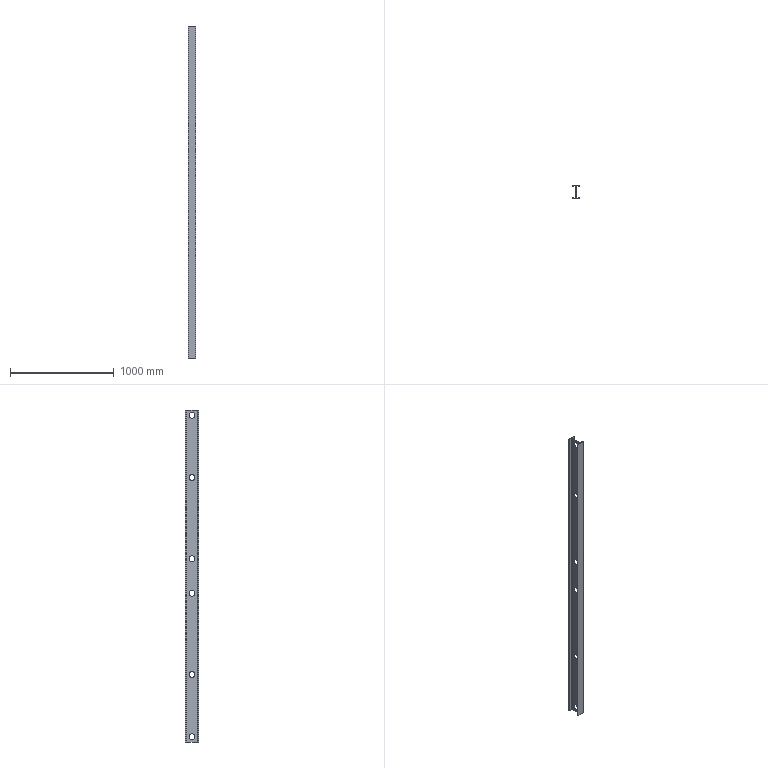Part | SolidWorks | features Extrusion 1, ICE 1 | 1 solid | 30 faces | box 74 x 126 x 3200 mm | volume 4580786 mm3 | cylinder 20 | plane 10 | commonest cylinder face diameters 55 x12 7 x4 14 x4
STEP:
#1=CARTESIAN_POINT('',(-2.5,27.5,2550.));
#2=VERTEX_POINT('',#1);
#3=CARTESIAN_POINT('',(-2.5,-27.5,2550.));
#4=VERTEX_POINT('',#3);
#5=CARTESIAN_POINT('',(-2.5,0.,2550.));
#6=DIRECTION('',(-1.,0.,0.));
#7=DIRECTION('',(0.,0.,-1.));
#8=AXIS2_PLACEMENT_3D('',#5,#6,#7);
#9=CIRCLE('',#8,27.5);
#10=EDGE_CURVE('',#2,#4,#9,.T.);
#11=ORIENTED_EDGE('',*,*,#10,.T.);
#12=CARTESIAN_POINT('',(2.5,-27.5,2550.));
#13=VERTEX_POINT('',#12);
#14=CARTESIAN_POINT('',(-37.001,-27.5,2550.));
#15=DIRECTION('',(1.,0.,0.));
#16=VECTOR('',#15,1000.);
#17=LINE('',#14,#16);
#18=EDGE_CURVE('',#4,#13,#17,.T.);
#19=ORIENTED_EDGE('',*,*,#18,.T.);
#20=CARTESIAN_POINT('',(2.5,27.5,2550.));
#21=VERTEX_POINT('',#20);
#22=CARTESIAN_POINT('',(2.5,0.,2550.));
#23=DIRECTION('',(1.,0.,0.));
#24=DIRECTION('',(0.,1.,0.));
#25=AXIS2_PLACEMENT_3D('',#22,#23,#24);
#26=CIRCLE('',#25,27.5);
#27=EDGE_CURVE('',#13,#21,#26,.T.);
#28=ORIENTED_EDGE('',*,*,#27,.T.);
#29=CARTESIAN_POINT('',(-37.001,27.5,2550.));
#30=DIRECTION('',(1.,0.,0.));
#31=VECTOR('',#30,1000.);
#32=LINE('',#29,#31);
#33=EDGE_CURVE('',#2,#21,#32,.T.);
#34=ORIENTED_EDGE('',*,*,#33,.F.);
#35=EDGE_LOOP('',(#11,#19,#28,#34));
#36=FACE_OUTER_BOUND('',#35,.T.);
#37=CARTESIAN_POINT('',(-37.001,0.,2550.));
#38=DIRECTION('',(1.,0.,0.));
#39=DIRECTION('',(0.,1.,0.));
#40=AXIS2_PLACEMENT_3D('',#37,#38,#39);
#41=CYLINDRICAL_SURFACE('',#40,27.5);
#42=ADVANCED_FACE('',(#36),#41,.F.);
#43=CARTESIAN_POINT('',(-2.5,27.5,3150.));
#44=VERTEX_POINT('',#43);
#45=CARTESIAN_POINT('',(-2.5,-27.5,3150.));
#46=VERTEX_POINT('',#45);
#47=CARTESIAN_POINT('',(-2.5,0.,3150.));
#48=DIRECTION('',(-1.,0.,0.));
#49=DIRECTION('',(0.,0.,-1.));
#50=AXIS2_PLACEMENT_3D('',#47,#48,#49);
#51=CIRCLE('',#50,27.5);
#52=EDGE_CURVE('',#44,#46,#51,.T.);
#53=ORIENTED_EDGE('',*,*,#52,.T.);
#54=CARTESIAN_POINT('',(2.5,-27.5,3150.));
#55=VERTEX_POINT('',#54);
#56=CARTESIAN_POINT('',(-37.001,-27.5,3150.));
#57=DIRECTION('',(1.,0.,0.));
#58=VECTOR('',#57,1000.);
#59=LINE('',#56,#58);
#60=EDGE_CURVE('',#46,#55,#59,.T.);
#61=ORIENTED_EDGE('',*,*,#60,.T.);
#62=CARTESIAN_POINT('',(2.5,27.5,3150.));
#63=VERTEX_POINT('',#62);
#64=CARTESIAN_POINT('',(2.5,0.,3150.));
#65=DIRECTION('',(1.,0.,0.));
#66=DIRECTION('',(0.,1.,0.));
#67=AXIS2_PLACEMENT_3D('',#64,#65,#66);
#68=CIRCLE('',#67,27.5);
#69=EDGE_CURVE('',#55,#63,#68,.T.);
#70=ORIENTED_EDGE('',*,*,#69,.T.);
#71=CARTESIAN_POINT('',(-37.001,27.5,3150.));
#72=DIRECTION('',(1.,0.,0.));
#73=VECTOR('',#72,1000.);
#74=LINE('',#71,#73);
#75=EDGE_CURVE('',#44,#63,#74,.T.);
#76=ORIENTED_EDGE('',*,*,#75,.F.);
#77=EDGE_LOOP('',(#53,#61,#70,#76));
#78=FACE_OUTER_BOUND('',#77,.T.);
#79=CARTESIAN_POINT('',(-37.001,0.,3150.));
#80=DIRECTION('',(1.,0.,0.));
#81=DIRECTION('',(0.,1.,0.));
#82=AXIS2_PLACEMENT_3D('',#79,#80,#81);
#83=CYLINDRICAL_SURFACE('',#82,27.5);
#84=ADVANCED_FACE('',(#78),#83,.F.);
#85=CARTESIAN_POINT('',(-2.5,27.5,1766.));
#86=VERTEX_POINT('',#85);
#87=CARTESIAN_POINT('',(-2.5,-27.5,1766.));
#88=VERTEX_POINT('',#87);
#89=CARTESIAN_POINT('',(-2.5,0.,1766.));
#90=DIRECTION('',(-1.,0.,0.));
#91=DIRECTION('',(0.,0.,-1.));
#92=AXIS2_PLACEMENT_3D('',#89,#90,#91);
#93=CIRCLE('',#92,27.5);
#94=EDGE_CURVE('',#86,#88,#93,.T.);
#95=ORIENTED_EDGE('',*,*,#94,.T.);
#96=CARTESIAN_POINT('',(2.5,-27.5,1766.));
#97=VERTEX_POINT('',#96);
#98=CARTESIAN_POINT('',(-37.001,-27.5,1766.));
#99=DIRECTION('',(1.,0.,0.));
#100=VECTOR('',#99,1000.);
#101=LINE('',#98,#100);
#102=EDGE_CURVE('',#88,#97,#101,.T.);
#103=ORIENTED_EDGE('',*,*,#102,.T.);
#104=CARTESIAN_POINT('',(2.5,27.5,1766.));
#105=VERTEX_POINT('',#104);
#106=CARTESIAN_POINT('',(2.5,0.,1766.));
#107=DIRECTION('',(1.,0.,0.));
#108=DIRECTION('',(0.,1.,0.));
#109=AXIS2_PLACEMENT_3D('',#106,#107,#108);
#110=CIRCLE('',#109,27.5);
#111=EDGE_CURVE('',#97,#105,#110,.T.);
#112=ORIENTED_EDGE('',*,*,#111,.T.);
#113=CARTESIAN_POINT('',(-37.001,27.5,1766.));
#114=DIRECTION('',(1.,0.,0.));
#115=VECTOR('',#114,1000.);
#116=LINE('',#113,#115);
#117=EDGE_CURVE('',#86,#105,#116,.T.);
#118=ORIENTED_EDGE('',*,*,#117,.F.);
#119=EDGE_LOOP('',(#95,#103,#112,#118));
#120=FACE_OUTER_BOUND('',#119,.T.);
#121=CARTESIAN_POINT('',(-37.001,0.,1766.));
#122=DIRECTION('',(1.,0.,0.));
#123=DIRECTION('',(0.,1.,0.));
#124=AXIS2_PLACEMENT_3D('',#121,#122,#123);
#125=CYLINDRICAL_SURFACE('',#124,27.5);
#126=ADVANCED_FACE('',(#120),#125,.F.);
#127=CARTESIAN_POINT('',(-2.5,27.5,1434.));
#128=VERTEX_POINT('',#127);
#129=CARTESIAN_POINT('',(-2.5,-27.5,1434.));
#130=VERTEX_POINT('',#129);
#131=CARTESIAN_POINT('',(-2.5,0.,1434.));
#132=DIRECTION('',(-1.,0.,0.));
#133=DIRECTION('',(0.,0.,-1.));
#134=AXIS2_PLACEMENT_3D('',#131,#132,#133);
#135=CIRCLE('',#134,27.5);
#136=EDGE_CURVE('',#128,#130,#135,.T.);
#137=ORIENTED_EDGE('',*,*,#136,.T.);
#138=CARTESIAN_POINT('',(2.5,-27.5,1434.));
#139=VERTEX_POINT('',#138);
#140=CARTESIAN_POINT('',(-37.001,-27.5,1434.));
#141=DIRECTION('',(1.,0.,0.));
#142=VECTOR('',#141,1000.);
#143=LINE('',#140,#142);
#144=EDGE_CURVE('',#130,#139,#143,.T.);
#145=ORIENTED_EDGE('',*,*,#144,.T.);
#146=CARTESIAN_POINT('',(2.5,27.5,1434.));
#147=VERTEX_POINT('',#146);
#148=CARTESIAN_POINT('',(2.5,0.,1434.));
#149=DIRECTION('',(1.,0.,0.));
#150=DIRECTION('',(0.,1.,0.));
#151=AXIS2_PLACEMENT_3D('',#148,#149,#150);
#152=CIRCLE('',#151,27.5);
#153=EDGE_CURVE('',#139,#147,#152,.T.);
#154=ORIENTED_EDGE('',*,*,#153,.T.);
#155=CARTESIAN_POINT('',(-37.001,27.5,1434.));
#156=DIRECTION('',(1.,0.,0.));
#157=VECTOR('',#156,1000.);
#158=LINE('',#155,#157);
#159=EDGE_CURVE('',#128,#147,#158,.T.);
#160=ORIENTED_EDGE('',*,*,#159,.F.);
#161=EDGE_LOOP('',(#137,#145,#154,#160));
#162=FACE_OUTER_BOUND('',#161,.T.);
#163=CARTESIAN_POINT('',(-37.001,0.,1434.));
#164=DIRECTION('',(1.,0.,0.));
#165=DIRECTION('',(0.,1.,0.));
#166=AXIS2_PLACEMENT_3D('',#163,#164,#165);
#167=CYLINDRICAL_SURFACE('',#166,27.5);
#168=ADVANCED_FACE('',(#162),#167,.F.);
#169=CARTESIAN_POINT('',(-2.5,27.5,650.));
#170=VERTEX_POINT('',#169);
#171=CARTESIAN_POINT('',(-2.5,-27.5,650.));
#172=VERTEX_POINT('',#171);
#173=CARTESIAN_POINT('',(-2.5,0.,650.));
#174=DIRECTION('',(-1.,0.,0.));
#175=DIRECTION('',(0.,0.,-1.));
#176=AXIS2_PLACEMENT_3D('',#173,#174,#175);
#177=CIRCLE('',#176,27.5);
#178=EDGE_CURVE('',#170,#172,#177,.T.);
#179=ORIENTED_EDGE('',*,*,#178,.T.);
#180=CARTESIAN_POINT('',(2.5,-27.5,650.));
#181=VERTEX_POINT('',#180);
#182=CARTESIAN_POINT('',(-37.001,-27.5,650.));
#183=DIRECTION('',(1.,0.,0.));
#184=VECTOR('',#183,1000.);
#185=LINE('',#182,#184);
#186=EDGE_CURVE('',#172,#181,#185,.T.);
#187=ORIENTED_EDGE('',*,*,#186,.T.);
#188=CARTESIAN_POINT('',(2.5,27.5,650.));
#189=VERTEX_POINT('',#188);
#190=CARTESIAN_POINT('',(2.5,0.,650.));
#191=DIRECTION('',(1.,0.,0.));
#192=DIRECTION('',(0.,1.,0.));
#193=AXIS2_PLACEMENT_3D('',#190,#191,#192);
#194=CIRCLE('',#193,27.5);
#195=EDGE_CURVE('',#181,#189,#194,.T.);
#196=ORIENTED_EDGE('',*,*,#195,.T.);
#197=CARTESIAN_POINT('',(-37.001,27.5,650.));
#198=DIRECTION('',(1.,0.,0.));
#199=VECTOR('',#198,1000.);
#200=LINE('',#197,#199);
#201=EDGE_CURVE('',#170,#189,#200,.T.);
#202=ORIENTED_EDGE('',*,*,#201,.F.);
#203=EDGE_LOOP('',(#179,#187,#196,#202));
#204=FACE_OUTER_BOUND('',#203,.T.);
#205=CARTESIAN_POINT('',(-37.001,0.,650.));
#206=DIRECTION('',(1.,0.,0.));
#207=DIRECTION('',(0.,1.,0.));
#208=AXIS2_PLACEMENT_3D('',#205,#206,#207);
#209=CYLINDRICAL_SURFACE('',#208,27.5);
#210=ADVANCED_FACE('',(#204),#209,.F.);
#211=CARTESIAN_POINT('',(-2.5,27.5,50.));
#212=VERTEX_POINT('',#211);
#213=CARTESIAN_POINT('',(-2.5,-27.5,50.));
#214=VERTEX_POINT('',#213);
#215=CARTESIAN_POINT('',(-2.5,0.,50.));
#216=DIRECTION('',(-1.,0.,0.));
#217=DIRECTION('',(0.,0.,-1.));
#218=AXIS2_PLACEMENT_3D('',#215,#216,#217);
#219=CIRCLE('',#218,27.5);
#220=EDGE_CURVE('',#212,#214,#219,.T.);
#221=ORIENTED_EDGE('',*,*,#220,.T.);
#222=CARTESIAN_POINT('',(2.5,-27.5,50.));
#223=VERTEX_POINT('',#222);
#224=CARTESIAN_POINT('',(-37.001,-27.5,50.));
#225=DIRECTION('',(1.,0.,0.));
#226=VECTOR('',#225,1000.);
#227=LINE('',#224,#226);
#228=EDGE_CURVE('',#214,#223,#227,.T.);
#229=ORIENTED_EDGE('',*,*,#228,.T.);
#230=CARTESIAN_POINT('',(2.5,27.5,50.));
#231=VERTEX_POINT('',#230);
#232=CARTESIAN_POINT('',(2.5,0.,50.));
#233=DIRECTION('',(1.,0.,0.));
#234=DIRECTION('',(0.,1.,0.));
#235=AXIS2_PLACEMENT_3D('',#232,#233,#234);
#236=CIRCLE('',#235,27.5);
#237=EDGE_CURVE('',#223,#231,#236,.T.);
#238=ORIENTED_EDGE('',*,*,#237,.T.);
#239=CARTESIAN_POINT('',(-37.001,27.5,50.));
#240=DIRECTION('',(1.,0.,0.));
#241=VECTOR('',#240,1000.);
#242=LINE('',#239,#241);
#243=EDGE_CURVE('',#212,#231,#242,.T.);
#244=ORIENTED_EDGE('',*,*,#243,.F.);
#245=EDGE_LOOP('',(#221,#229,#238,#244));
#246=FACE_OUTER_BOUND('',#245,.T.);
#247=CARTESIAN_POINT('',(-37.001,0.,50.));
#248=DIRECTION('',(1.,0.,0.));
#249=DIRECTION('',(0.,1.,0.));
#250=AXIS2_PLACEMENT_3D('',#247,#248,#249);
#251=CYLINDRICAL_SURFACE('',#250,27.5);
#252=ADVANCED_FACE('',(#246),#251,.F.);
#253=CARTESIAN_POINT('',(-2.5,-48.4,0.));
#254=VERTEX_POINT('',#253);
#255=CARTESIAN_POINT('',(-8.361,-55.307,0.));
#256=VERTEX_POINT('',#255);
#257=CARTESIAN_POINT('',(-9.5,-48.4,0.));
#258=DIRECTION('',(0.,0.,-1.));
#259=DIRECTION('',(-1.,0.,0.));
#260=AXIS2_PLACEMENT_3D('',#257,#258,#259);
#261=CIRCLE('',#260,7.);
#262=EDGE_CURVE('',#254,#256,#261,.T.);
#263=ORIENTED_EDGE('',*,*,#262,.T.);
#264=CARTESIAN_POINT('',(-8.361,-55.307,3200.));
#265=VERTEX_POINT('',#264);
#266=CARTESIAN_POINT('',(-8.361,-55.307,3200.));
#267=DIRECTION('',(0.,0.,-1.));
#268=VECTOR('',#267,1000.);
#269=LINE('',#266,#268);
#270=EDGE_CURVE('',#265,#256,#269,.T.);
#271=ORIENTED_EDGE('',*,*,#270,.F.);
#272=CARTESIAN_POINT('',(-2.5,-48.4,3200.));
#273=VERTEX_POINT('',#272);
#274=CARTESIAN_POINT('',(-9.5,-48.4,3200.));
#275=DIRECTION('',(0.,0.,-1.));
#276=DIRECTION('',(-1.,0.,0.));
#277=AXIS2_PLACEMENT_3D('',#274,#275,#276);
#278=CIRCLE('',#277,7.);
#279=EDGE_CURVE('',#273,#265,#278,.T.);
#280=ORIENTED_EDGE('',*,*,#279,.F.);
#281=CARTESIAN_POINT('',(-2.5,-48.4,3200.));
#282=DIRECTION('',(0.,0.,-1.));
#283=VECTOR('',#282,1000.);
#284=LINE('',#281,#283);
#285=EDGE_CURVE('',#273,#254,#284,.T.);
#286=ORIENTED_EDGE('',*,*,#285,.T.);
#287=EDGE_LOOP('',(#263,#271,#280,#286));
#288=FACE_OUTER_BOUND('',#287,.T.);
#289=CARTESIAN_POINT('',(-9.5,-48.4,3200.));
#290=DIRECTION('',(0.,0.,-1.));
#291=DIRECTION('',(-1.,0.,0.));
#292=AXIS2_PLACEMENT_3D('',#289,#290,#291);
#293=CYLINDRICAL_SURFACE('',#292,7.);
#294=ADVANCED_FACE('',(#288),#293,.F.);
#295=CARTESIAN_POINT('',(-34.07,-59.547,0.));
#296=VERTEX_POINT('',#295);
#297=CARTESIAN_POINT('',(-34.07,-59.547,0.));
#298=DIRECTION('',(-0.9867,-0.1627,0.));
#299=VECTOR('',#298,1000.);
#300=LINE('',#297,#299);
#301=EDGE_CURVE('',#256,#296,#300,.T.);
#302=ORIENTED_EDGE('',*,*,#301,.T.);
#303=CARTESIAN_POINT('',(-34.07,-59.547,3200.));
#304=VERTEX_POINT('',#303);
#305=CARTESIAN_POINT('',(-34.07,-59.547,3200.));
#306=DIRECTION('',(0.,0.,-1.));
#307=VECTOR('',#306,1000.);
#308=LINE('',#305,#307);
#309=EDGE_CURVE('',#304,#296,#308,.T.);
#310=ORIENTED_EDGE('',*,*,#309,.F.);
#311=CARTESIAN_POINT('',(-34.07,-59.547,3200.));
#312=DIRECTION('',(-0.9867,-0.1627,0.));
#313=VECTOR('',#312,1000.);
#314=LINE('',#311,#313);
#315=EDGE_CURVE('',#265,#304,#314,.T.);
#316=ORIENTED_EDGE('',*,*,#315,.F.);
#317=ORIENTED_EDGE('',*,*,#270,.T.);
#318=EDGE_LOOP('',(#302,#310,#316,#317));
#319=FACE_OUTER_BOUND('',#318,.T.);
#320=CARTESIAN_POINT('',(-34.07,-59.547,3200.));
#321=DIRECTION('',(0.1627,-0.9867,0.));
#322=DIRECTION('',(0.9867,0.1627,0.));
#323=AXIS2_PLACEMENT_3D('',#320,#321,#322);
#324=PLANE('',#323);
#325=ADVANCED_FACE('',(#319),#324,.F.);
#326=CARTESIAN_POINT('',(-37.,-63.,0.));
#327=VERTEX_POINT('',#326);
#328=CARTESIAN_POINT('',(-33.5,-63.,0.));
#329=DIRECTION('',(0.,0.,1.));
#330=DIRECTION('',(-1.,0.,0.));
#331=AXIS2_PLACEMENT_3D('',#328,#329,#330);
#332=CIRCLE('',#331,3.5);
#333=EDGE_CURVE('',#296,#327,#332,.T.);
#334=ORIENTED_EDGE('',*,*,#333,.T.);
#335=CARTESIAN_POINT('',(-37.,-63.,3200.));
#336=VERTEX_POINT('',#335);
#337=CARTESIAN_POINT('',(-37.,-63.,3200.));
#338=DIRECTION('',(0.,0.,-1.));
#339=VECTOR('',#338,1000.);
#340=LINE('',#337,#339);
#341=EDGE_CURVE('',#336,#327,#340,.T.);
#342=ORIENTED_EDGE('',*,*,#341,.F.);
#343=CARTESIAN_POINT('',(-33.5,-63.,3200.));
#344=DIRECTION('',(0.,0.,1.));
#345=DIRECTION('',(-1.,0.,0.));
#346=AXIS2_PLACEMENT_3D('',#343,#344,#345);
#347=CIRCLE('',#346,3.5);
#348=EDGE_CURVE('',#304,#336,#347,.T.);
#349=ORIENTED_EDGE('',*,*,#348,.F.);
#350=ORIENTED_EDGE('',*,*,#309,.T.);
#351=EDGE_LOOP('',(#334,#342,#349,#350));
#352=FACE_OUTER_BOUND('',#351,.T.);
#353=CARTESIAN_POINT('',(-33.5,-63.,3200.));
#354=DIRECTION('',(0.,0.,-1.));
#355=DIRECTION('',(-1.,0.,0.));
#356=AXIS2_PLACEMENT_3D('',#353,#354,#355);
#357=CYLINDRICAL_SURFACE('',#356,3.5);
#358=ADVANCED_FACE('',(#352),#357,.T.);
#359=CARTESIAN_POINT('',(37.,-63.,0.));
#360=VERTEX_POINT('',#359);
#361=CARTESIAN_POINT('',(-37.,-63.,0.));
#362=DIRECTION('',(1.,0.,0.));
#363=VECTOR('',#362,1000.);
#364=LINE('',#361,#363);
#365=EDGE_CURVE('',#327,#360,#364,.T.);
#366=ORIENTED_EDGE('',*,*,#365,.T.);
#367=CARTESIAN_POINT('',(37.,-63.,3200.));
#368=VERTEX_POINT('',#367);
#369=CARTESIAN_POINT('',(37.,-63.,3200.));
#370=DIRECTION('',(0.,0.,-1.));
#371=VECTOR('',#370,1000.);
#372=LINE('',#369,#371);
#373=EDGE_CURVE('',#368,#360,#372,.T.);
#374=ORIENTED_EDGE('',*,*,#373,.F.);
#375=CARTESIAN_POINT('',(-37.,-63.,3200.));
#376=DIRECTION('',(1.,0.,0.));
#377=VECTOR('',#376,1000.);
#378=LINE('',#375,#377);
#379=EDGE_CURVE('',#336,#368,#378,.T.);
#380=ORIENTED_EDGE('',*,*,#379,.F.);
#381=ORIENTED_EDGE('',*,*,#341,.T.);
#382=EDGE_LOOP('',(#366,#374,#380,#381));
#383=FACE_OUTER_BOUND('',#382,.T.);
#384=CARTESIAN_POINT('',(-37.,-63.,3200.));
#385=DIRECTION('',(0.,1.,0.));
#386=DIRECTION('',(0.,0.,1.));
#387=AXIS2_PLACEMENT_3D('',#384,#385,#386);
#388=PLANE('',#387);
#389=ADVANCED_FACE('',(#383),#388,.F.);
#390=CARTESIAN_POINT('',(34.07,-59.547,0.));
#391=VERTEX_POINT('',#390);
#392=CARTESIAN_POINT('',(33.5,-63.,0.));
#393=DIRECTION('',(0.,0.,1.));
#394=DIRECTION('',(1.,0.,0.));
#395=AXIS2_PLACEMENT_3D('',#392,#393,#394);
#396=CIRCLE('',#395,3.5);
#397=EDGE_CURVE('',#360,#391,#396,.T.);
#398=ORIENTED_EDGE('',*,*,#397,.T.);
#399=CARTESIAN_POINT('',(34.07,-59.547,3200.));
#400=VERTEX_POINT('',#399);
#401=CARTESIAN_POINT('',(34.07,-59.547,3200.));
#402=DIRECTION('',(0.,0.,-1.));
#403=VECTOR('',#402,1000.);
#404=LINE('',#401,#403);
#405=EDGE_CURVE('',#400,#391,#404,.T.);
#406=ORIENTED_EDGE('',*,*,#405,.F.);
#407=CARTESIAN_POINT('',(33.5,-63.,3200.));
#408=DIRECTION('',(0.,0.,1.));
#409=DIRECTION('',(1.,0.,0.));
#410=AXIS2_PLACEMENT_3D('',#407,#408,#409);
#411=CIRCLE('',#410,3.5);
#412=EDGE_CURVE('',#368,#400,#411,.T.);
#413=ORIENTED_EDGE('',*,*,#412,.F.);
#414=ORIENTED_EDGE('',*,*,#373,.T.);
#415=EDGE_LOOP('',(#398,#406,#413,#414));
#416=FACE_OUTER_BOUND('',#415,.T.);
#417=CARTESIAN_POINT('',(33.5,-63.,3200.));
#418=DIRECTION('',(0.,0.,-1.));
#419=DIRECTION('',(-1.,0.,0.));
#420=AXIS2_PLACEMENT_3D('',#417,#418,#419);
#421=CYLINDRICAL_SURFACE('',#420,3.5);
#422=ADVANCED_FACE('',(#416),#421,.T.);
#423=CARTESIAN_POINT('',(8.361,-55.307,0.));
#424=VERTEX_POINT('',#423);
#425=CARTESIAN_POINT('',(34.07,-59.547,0.));
#426=DIRECTION('',(-0.9867,0.1627,0.));
#427=VECTOR('',#426,1000.);
#428=LINE('',#425,#427);
#429=EDGE_CURVE('',#391,#424,#428,.T.);
#430=ORIENTED_EDGE('',*,*,#429,.T.);
#431=CARTESIAN_POINT('',(8.361,-55.307,3200.));
#432=VERTEX_POINT('',#431);
#433=CARTESIAN_POINT('',(8.361,-55.307,3200.));
#434=DIRECTION('',(0.,0.,-1.));
#435=VECTOR('',#434,1000.);
#436=LINE('',#433,#435);
#437=EDGE_CURVE('',#432,#424,#436,.T.);
#438=ORIENTED_EDGE('',*,*,#437,.F.);
#439=CARTESIAN_POINT('',(34.07,-59.547,3200.));
#440=DIRECTION('',(-0.9867,0.1627,0.));
#441=VECTOR('',#440,1000.);
#442=LINE('',#439,#441);
#443=EDGE_CURVE('',#400,#432,#442,.T.);
#444=ORIENTED_EDGE('',*,*,#443,.F.);
#445=ORIENTED_EDGE('',*,*,#405,.T.);
#446=EDGE_LOOP('',(#430,#438,#444,#445));
#447=FACE_OUTER_BOUND('',#446,.T.);
#448=CARTESIAN_POINT('',(34.07,-59.547,3200.));
#449=DIRECTION('',(-0.1627,-0.9867,0.));
#450=DIRECTION('',(0.9867,-0.1627,0.));
#451=AXIS2_PLACEMENT_3D('',#448,#449,#450);
#452=PLANE('',#451);
#453=ADVANCED_FACE('',(#447),#452,.F.);
#454=CARTESIAN_POINT('',(2.5,-48.4,0.));
#455=VERTEX_POINT('',#454);
#456=CARTESIAN_POINT('',(9.5,-48.4,0.));
#457=DIRECTION('',(0.,0.,-1.));
#458=DIRECTION('',(1.,0.,0.));
#459=AXIS2_PLACEMENT_3D('',#456,#457,#458);
#460=CIRCLE('',#459,7.);
#461=EDGE_CURVE('',#424,#455,#460,.T.);
#462=ORIENTED_EDGE('',*,*,#461,.T.);
#463=CARTESIAN_POINT('',(2.5,-48.4,3200.));
#464=VERTEX_POINT('',#463);
#465=CARTESIAN_POINT('',(2.5,-48.4,3200.));
#466=DIRECTION('',(0.,0.,-1.));
#467=VECTOR('',#466,1000.);
#468=LINE('',#465,#467);
#469=EDGE_CURVE('',#464,#455,#468,.T.);
#470=ORIENTED_EDGE('',*,*,#469,.F.);
#471=CARTESIAN_POINT('',(9.5,-48.4,3200.));
#472=DIRECTION('',(0.,0.,-1.));
#473=DIRECTION('',(1.,0.,0.));
#474=AXIS2_PLACEMENT_3D('',#471,#472,#473);
#475=CIRCLE('',#474,7.);
#476=EDGE_CURVE('',#432,#464,#475,.T.);
#477=ORIENTED_EDGE('',*,*,#476,.F.);
#478=ORIENTED_EDGE('',*,*,#437,.T.);
#479=EDGE_LOOP('',(#462,#470,#477,#478));
#480=FACE_OUTER_BOUND('',#479,.T.);
#481=CARTESIAN_POINT('',(9.5,-48.4,3200.));
#482=DIRECTION('',(0.,0.,-1.));
#483=DIRECTION('',(-1.,0.,0.));
#484=AXIS2_PLACEMENT_3D('',#481,#482,#483);
#485=CYLINDRICAL_SURFACE('',#484,7.);
#486=ADVANCED_FACE('',(#480),#485,.F.);
#487=CARTESIAN_POINT('',(2.5,0.,2550.));
#488=DIRECTION('',(1.,0.,0.));
#489=DIRECTION('',(0.,1.,0.));
#490=AXIS2_PLACEMENT_3D('',#487,#488,#489);
#491=CIRCLE('',#490,27.5);
#492=EDGE_CURVE('',#21,#13,#491,.T.);
#493=ORIENTED_EDGE('',*,*,#492,.F.);
#494=ORIENTED_EDGE('',*,*,#27,.F.);
#495=EDGE_LOOP('',(#493,#494));
#496=FACE_BOUND('',#495,.T.);
#497=CARTESIAN_POINT('',(2.5,0.,3150.));
#498=DIRECTION('',(1.,0.,0.));
#499=DIRECTION('',(0.,1.,0.));
#500=AXIS2_PLACEMENT_3D('',#497,#498,#499);
#501=CIRCLE('',#500,27.5);
#502=EDGE_CURVE('',#63,#55,#501,.T.);
#503=ORIENTED_EDGE('',*,*,#502,.F.);
#504=ORIENTED_EDGE('',*,*,#69,.F.);
#505=EDGE_LOOP('',(#503,#504));
#506=FACE_BOUND('',#505,.T.);
#507=CARTESIAN_POINT('',(2.5,0.,1766.));
#508=DIRECTION('',(1.,0.,0.));
#509=DIRECTION('',(0.,1.,0.));
#510=AXIS2_PLACEMENT_3D('',#507,#508,#509);
#511=CIRCLE('',#510,27.5);
#512=EDGE_CURVE('',#105,#97,#511,.T.);
#513=ORIENTED_EDGE('',*,*,#512,.F.);
#514=ORIENTED_EDGE('',*,*,#111,.F.);
#515=EDGE_LOOP('',(#513,#514));
#516=FACE_BOUND('',#515,.T.);
#517=CARTESIAN_POINT('',(2.5,0.,1434.));
#518=DIRECTION('',(1.,0.,0.));
#519=DIRECTION('',(0.,1.,0.));
#520=AXIS2_PLACEMENT_3D('',#517,#518,#519);
#521=CIRCLE('',#520,27.5);
#522=EDGE_CURVE('',#147,#139,#521,.T.);
#523=ORIENTED_EDGE('',*,*,#522,.F.);
#524=ORIENTED_EDGE('',*,*,#153,.F.);
#525=EDGE_LOOP('',(#523,#524));
#526=FACE_BOUND('',#525,.T.);
#527=CARTESIAN_POINT('',(2.5,0.,650.));
#528=DIRECTION('',(1.,0.,0.));
#529=DIRECTION('',(0.,1.,0.));
#530=AXIS2_PLACEMENT_3D('',#527,#528,#529);
#531=CIRCLE('',#530,27.5);
#532=EDGE_CURVE('',#189,#181,#531,.T.);
#533=ORIENTED_EDGE('',*,*,#532,.F.);
#534=ORIENTED_EDGE('',*,*,#195,.F.);
#535=EDGE_LOOP('',(#533,#534));
#536=FACE_BOUND('',#535,.T.);
#537=CARTESIAN_POINT('',(2.5,0.,50.));
#538=DIRECTION('',(1.,0.,0.));
#539=DIRECTION('',(0.,1.,0.));
#540=AXIS2_PLACEMENT_3D('',#537,#538,#539);
#541=CIRCLE('',#540,27.5);
#542=EDGE_CURVE('',#231,#223,#541,.T.);
#543=ORIENTED_EDGE('',*,*,#542,.F.);
#544=ORIENTED_EDGE('',*,*,#237,.F.);
#545=EDGE_LOOP('',(#543,#544));
#546=FACE_BOUND('',#545,.T.);
#547=CARTESIAN_POINT('',(2.5,48.4,0.));
#548=VERTEX_POINT('',#547);
#549=CARTESIAN_POINT('',(2.5,48.4,0.));
#550=DIRECTION('',(0.,1.,0.));
#551=VECTOR('',#550,1000.);
#552=LINE('',#549,#551);
#553=EDGE_CURVE('',#455,#548,#552,.T.);
#554=ORIENTED_EDGE('',*,*,#553,.T.);
#555=CARTESIAN_POINT('',(2.5,48.4,3200.));
#556=VERTEX_POINT('',#555);
#557=CARTESIAN_POINT('',(2.5,48.4,3200.));
#558=DIRECTION('',(0.,0.,-1.));
#559=VECTOR('',#558,1000.);
#560=LINE('',#557,#559);
#561=EDGE_CURVE('',#556,#548,#560,.T.);
#562=ORIENTED_EDGE('',*,*,#561,.F.);
#563=CARTESIAN_POINT('',(2.5,48.4,3200.));
#564=DIRECTION('',(0.,1.,0.));
#565=VECTOR('',#564,1000.);
#566=LINE('',#563,#565);
#567=EDGE_CURVE('',#464,#556,#566,.T.);
#568=ORIENTED_EDGE('',*,*,#567,.F.);
#569=ORIENTED_EDGE('',*,*,#469,.T.);
#570=EDGE_LOOP('',(#554,#562,#568,#569));
#571=FACE_OUTER_BOUND('',#570,.T.);
#572=CARTESIAN_POINT('',(2.5,48.4,3200.));
#573=DIRECTION('',(-1.,0.,0.));
#574=DIRECTION('',(0.,-1.,0.));
#575=AXIS2_PLACEMENT_3D('',#572,#573,#574);
#576=PLANE('',#575);
#577=ADVANCED_FACE('',(#496,#506,#516,#526,#536,#546,#571),#576,.F.);
#578=CARTESIAN_POINT('',(8.361,55.307,0.));
#579=VERTEX_POINT('',#578);
#580=CARTESIAN_POINT('',(9.5,48.4,0.));
#581=DIRECTION('',(0.,0.,-1.));
#582=DIRECTION('',(-1.,0.,0.));
#583=AXIS2_PLACEMENT_3D('',#580,#581,#582);
#584=CIRCLE('',#583,7.);
#585=EDGE_CURVE('',#548,#579,#584,.T.);
#586=ORIENTED_EDGE('',*,*,#585,.T.);
#587=CARTESIAN_POINT('',(8.361,55.307,3200.));
#588=VERTEX_POINT('',#587);
#589=CARTESIAN_POINT('',(8.361,55.307,3200.));
#590=DIRECTION('',(0.,0.,-1.));
#591=VECTOR('',#590,1000.);
#592=LINE('',#589,#591);
#593=EDGE_CURVE('',#588,#579,#592,.T.);
#594=ORIENTED_EDGE('',*,*,#593,.F.);
#595=CARTESIAN_POINT('',(9.5,48.4,3200.));
#596=DIRECTION('',(0.,0.,-1.));
#597=DIRECTION('',(-1.,0.,0.));
#598=AXIS2_PLACEMENT_3D('',#595,#596,#597);
#599=CIRCLE('',#598,7.);
#600=EDGE_CURVE('',#556,#588,#599,.T.);
#601=ORIENTED_EDGE('',*,*,#600,.F.);
#602=ORIENTED_EDGE('',*,*,#561,.T.);
#603=EDGE_LOOP('',(#586,#594,#601,#602));
#604=FACE_OUTER_BOUND('',#603,.T.);
#605=CARTESIAN_POINT('',(9.5,48.4,3200.));
#606=DIRECTION('',(0.,0.,-1.));
#607=DIRECTION('',(-1.,0.,0.));
#608=AXIS2_PLACEMENT_3D('',#605,#606,#607);
#609=CYLINDRICAL_SURFACE('',#608,7.);
#610=ADVANCED_FACE('',(#604),#609,.F.);
#611=CARTESIAN_POINT('',(34.07,59.547,0.));
#612=VERTEX_POINT('',#611);
#613=CARTESIAN_POINT('',(34.07,59.547,0.));
#614=DIRECTION('',(0.9867,0.1627,0.));
#615=VECTOR('',#614,1000.);
#616=LINE('',#613,#615);
#617=EDGE_CURVE('',#579,#612,#616,.T.);
#618=ORIENTED_EDGE('',*,*,#617,.T.);
#619=CARTESIAN_POINT('',(34.07,59.547,3200.));
#620=VERTEX_POINT('',#619);
#621=CARTESIAN_POINT('',(34.07,59.547,3200.));
#622=DIRECTION('',(0.,0.,-1.));
#623=VECTOR('',#622,1000.);
#624=LINE('',#621,#623);
#625=EDGE_CURVE('',#620,#612,#624,.T.);
#626=ORIENTED_EDGE('',*,*,#625,.F.);
#627=CARTESIAN_POINT('',(34.07,59.547,3200.));
#628=DIRECTION('',(0.9867,0.1627,0.));
#629=VECTOR('',#628,1000.);
#630=LINE('',#627,#629);
#631=EDGE_CURVE('',#588,#620,#630,.T.);
#632=ORIENTED_EDGE('',*,*,#631,.F.);
#633=ORIENTED_EDGE('',*,*,#593,.T.);
#634=EDGE_LOOP('',(#618,#626,#632,#633));
#635=FACE_OUTER_BOUND('',#634,.T.);
#636=CARTESIAN_POINT('',(34.07,59.547,3200.));
#637=DIRECTION('',(-0.1627,0.9867,0.));
#638=DIRECTION('',(-0.9867,-0.1627,0.));
#639=AXIS2_PLACEMENT_3D('',#636,#637,#638);
#640=PLANE('',#639);
#641=ADVANCED_FACE('',(#635),#640,.F.);
#642=CARTESIAN_POINT('',(37.,63.,0.));
#643=VERTEX_POINT('',#642);
#644=CARTESIAN_POINT('',(33.5,63.,0.));
#645=DIRECTION('',(0.,0.,1.));
#646=DIRECTION('',(-1.,0.,0.));
#647=AXIS2_PLACEMENT_3D('',#644,#645,#646);
#648=CIRCLE('',#647,3.5);
#649=EDGE_CURVE('',#612,#643,#648,.T.);
#650=ORIENTED_EDGE('',*,*,#649,.T.);
#651=CARTESIAN_POINT('',(37.,63.,3200.));
#652=VERTEX_POINT('',#651);
#653=CARTESIAN_POINT('',(37.,63.,3200.));
#654=DIRECTION('',(0.,0.,-1.));
#655=VECTOR('',#654,1000.);
#656=LINE('',#653,#655);
#657=EDGE_CURVE('',#652,#643,#656,.T.);
#658=ORIENTED_EDGE('',*,*,#657,.F.);
#659=CARTESIAN_POINT('',(33.5,63.,3200.));
#660=DIRECTION('',(0.,0.,1.));
#661=DIRECTION('',(-1.,0.,0.));
#662=AXIS2_PLACEMENT_3D('',#659,#660,#661);
#663=CIRCLE('',#662,3.5);
#664=EDGE_CURVE('',#620,#652,#663,.T.);
#665=ORIENTED_EDGE('',*,*,#664,.F.);
#666=ORIENTED_EDGE('',*,*,#625,.T.);
#667=EDGE_LOOP('',(#650,#658,#665,#666));
#668=FACE_OUTER_BOUND('',#667,.T.);
#669=CARTESIAN_POINT('',(33.5,63.,3200.));
#670=DIRECTION('',(0.,0.,-1.));
#671=DIRECTION('',(-1.,0.,0.));
#672=AXIS2_PLACEMENT_3D('',#669,#670,#671);
#673=CYLINDRICAL_SURFACE('',#672,3.5);
#674=ADVANCED_FACE('',(#668),#673,.T.);
#675=CARTESIAN_POINT('',(-37.,63.,0.));
#676=VERTEX_POINT('',#675);
#677=CARTESIAN_POINT('',(-37.,63.,0.));
#678=DIRECTION('',(-1.,0.,0.));
#679=VECTOR('',#678,1000.);
#680=LINE('',#677,#679);
#681=EDGE_CURVE('',#643,#676,#680,.T.);
#682=ORIENTED_EDGE('',*,*,#681,.T.);
#683=CARTESIAN_POINT('',(-37.,63.,3200.));
#684=VERTEX_POINT('',#683);
#685=CARTESIAN_POINT('',(-37.,63.,3200.));
#686=DIRECTION('',(0.,0.,-1.));
#687=VECTOR('',#686,1000.);
#688=LINE('',#685,#687);
#689=EDGE_CURVE('',#684,#676,#688,.T.);
#690=ORIENTED_EDGE('',*,*,#689,.F.);
#691=CARTESIAN_POINT('',(-37.,63.,3200.));
#692=DIRECTION('',(-1.,0.,0.));
#693=VECTOR('',#692,1000.);
#694=LINE('',#691,#693);
#695=EDGE_CURVE('',#652,#684,#694,.T.);
#696=ORIENTED_EDGE('',*,*,#695,.F.);
#697=ORIENTED_EDGE('',*,*,#657,.T.);
#698=EDGE_LOOP('',(#682,#690,#696,#697));
#699=FACE_OUTER_BOUND('',#698,.T.);
#700=CARTESIAN_POINT('',(-37.,63.,3200.));
#701=DIRECTION('',(0.,-1.,0.));
#702=DIRECTION('',(0.,0.,-1.));
#703=AXIS2_PLACEMENT_3D('',#700,#701,#702);
#704=PLANE('',#703);
#705=ADVANCED_FACE('',(#699),#704,.F.);
#706=CARTESIAN_POINT('',(-34.07,59.547,0.));
#707=VERTEX_POINT('',#706);
#708=CARTESIAN_POINT('',(-33.5,63.,0.));
#709=DIRECTION('',(0.,0.,1.));
#710=DIRECTION('',(1.,0.,0.));
#711=AXIS2_PLACEMENT_3D('',#708,#709,#710);
#712=CIRCLE('',#711,3.5);
#713=EDGE_CURVE('',#676,#707,#712,.T.);
#714=ORIENTED_EDGE('',*,*,#713,.T.);
#715=CARTESIAN_POINT('',(-34.07,59.547,3200.));
#716=VERTEX_POINT('',#715);
#717=CARTESIAN_POINT('',(-34.07,59.547,3200.));
#718=DIRECTION('',(0.,0.,-1.));
#719=VECTOR('',#718,1000.);
#720=LINE('',#717,#719);
#721=EDGE_CURVE('',#716,#707,#720,.T.);
#722=ORIENTED_EDGE('',*,*,#721,.F.);
#723=CARTESIAN_POINT('',(-33.5,63.,3200.));
#724=DIRECTION('',(0.,0.,1.));
#725=DIRECTION('',(1.,0.,0.));
#726=AXIS2_PLACEMENT_3D('',#723,#724,#725);
#727=CIRCLE('',#726,3.5);
#728=EDGE_CURVE('',#684,#716,#727,.T.);
#729=ORIENTED_EDGE('',*,*,#728,.F.);
#730=ORIENTED_EDGE('',*,*,#689,.T.);
#731=EDGE_LOOP('',(#714,#722,#729,#730));
#732=FACE_OUTER_BOUND('',#731,.T.);
#733=CARTESIAN_POINT('',(-33.5,63.,3200.));
#734=DIRECTION('',(0.,0.,-1.));
#735=DIRECTION('',(-1.,0.,0.));
#736=AXIS2_PLACEMENT_3D('',#733,#734,#735);
#737=CYLINDRICAL_SURFACE('',#736,3.5);
#738=ADVANCED_FACE('',(#732),#737,.T.);
#739=CARTESIAN_POINT('',(-8.361,55.307,0.));
#740=VERTEX_POINT('',#739);
#741=CARTESIAN_POINT('',(-34.07,59.547,0.));
#742=DIRECTION('',(0.9867,-0.1627,0.));
#743=VECTOR('',#742,1000.);
#744=LINE('',#741,#743);
#745=EDGE_CURVE('',#707,#740,#744,.T.);
#746=ORIENTED_EDGE('',*,*,#745,.T.);
#747=CARTESIAN_POINT('',(-8.361,55.307,3200.));
#748=VERTEX_POINT('',#747);
#749=CARTESIAN_POINT('',(-8.361,55.307,3200.));
#750=DIRECTION('',(0.,0.,-1.));
#751=VECTOR('',#750,1000.);
#752=LINE('',#749,#751);
#753=EDGE_CURVE('',#748,#740,#752,.T.);
#754=ORIENTED_EDGE('',*,*,#753,.F.);
#755=CARTESIAN_POINT('',(-34.07,59.547,3200.));
#756=DIRECTION('',(0.9867,-0.1627,0.));
#757=VECTOR('',#756,1000.);
#758=LINE('',#755,#757);
#759=EDGE_CURVE('',#716,#748,#758,.T.);
#760=ORIENTED_EDGE('',*,*,#759,.F.);
#761=ORIENTED_EDGE('',*,*,#721,.T.);
#762=EDGE_LOOP('',(#746,#754,#760,#761));
#763=FACE_OUTER_BOUND('',#762,.T.);
#764=CARTESIAN_POINT('',(-34.07,59.547,3200.));
#765=DIRECTION('',(0.1627,0.9867,0.));
#766=DIRECTION('',(-0.9867,0.1627,0.));
#767=AXIS2_PLACEMENT_3D('',#764,#765,#766);
#768=PLANE('',#767);
#769=ADVANCED_FACE('',(#763),#768,.F.);
#770=CARTESIAN_POINT('',(-2.5,48.4,0.));
#771=VERTEX_POINT('',#770);
#772=CARTESIAN_POINT('',(-9.5,48.4,0.));
#773=DIRECTION('',(0.,0.,-1.));
#774=DIRECTION('',(1.,0.,0.));
#775=AXIS2_PLACEMENT_3D('',#772,#773,#774);
#776=CIRCLE('',#775,7.);
#777=EDGE_CURVE('',#740,#771,#776,.T.);
#778=ORIENTED_EDGE('',*,*,#777,.T.);
#779=CARTESIAN_POINT('',(-2.5,48.4,3200.));
#780=VERTEX_POINT('',#779);
#781=CARTESIAN_POINT('',(-2.5,48.4,3200.));
#782=DIRECTION('',(0.,0.,-1.));
#783=VECTOR('',#782,1000.);
#784=LINE('',#781,#783);
#785=EDGE_CURVE('',#780,#771,#784,.T.);
#786=ORIENTED_EDGE('',*,*,#785,.F.);
#787=CARTESIAN_POINT('',(-9.5,48.4,3200.));
#788=DIRECTION('',(0.,0.,-1.));
#789=DIRECTION('',(1.,0.,0.));
#790=AXIS2_PLACEMENT_3D('',#787,#788,#789);
#791=CIRCLE('',#790,7.);
#792=EDGE_CURVE('',#748,#780,#791,.T.);
#793=ORIENTED_EDGE('',*,*,#792,.F.);
#794=ORIENTED_EDGE('',*,*,#753,.T.);
#795=EDGE_LOOP('',(#778,#786,#793,#794));
#796=FACE_OUTER_BOUND('',#795,.T.);
#797=CARTESIAN_POINT('',(-9.5,48.4,3200.));
#798=DIRECTION('',(0.,0.,-1.));
#799=DIRECTION('',(-1.,0.,0.));
#800=AXIS2_PLACEMENT_3D('',#797,#798,#799);
#801=CYLINDRICAL_SURFACE('',#800,7.);
#802=ADVANCED_FACE('',(#796),#801,.F.);
#803=ORIENTED_EDGE('',*,*,#10,.F.);
#804=CARTESIAN_POINT('',(-2.5,0.,2550.));
#805=DIRECTION('',(-1.,0.,0.));
#806=DIRECTION('',(0.,0.,-1.));
#807=AXIS2_PLACEMENT_3D('',#804,#805,#806);
#808=CIRCLE('',#807,27.5);
#809=EDGE_CURVE('',#4,#2,#808,.T.);
#810=ORIENTED_EDGE('',*,*,#809,.F.);
#811=EDGE_LOOP('',(#803,#810));
#812=FACE_BOUND('',#811,.T.);
#813=ORIENTED_EDGE('',*,*,#52,.F.);
#814=CARTESIAN_POINT('',(-2.5,0.,3150.));
#815=DIRECTION('',(-1.,0.,0.));
#816=DIRECTION('',(0.,0.,-1.));
#817=AXIS2_PLACEMENT_3D('',#814,#815,#816);
#818=CIRCLE('',#817,27.5);
#819=EDGE_CURVE('',#46,#44,#818,.T.);
#820=ORIENTED_EDGE('',*,*,#819,.F.);
#821=EDGE_LOOP('',(#813,#820));
#822=FACE_BOUND('',#821,.T.);
#823=ORIENTED_EDGE('',*,*,#94,.F.);
#824=CARTESIAN_POINT('',(-2.5,0.,1766.));
#825=DIRECTION('',(-1.,0.,0.));
#826=DIRECTION('',(0.,0.,-1.));
#827=AXIS2_PLACEMENT_3D('',#824,#825,#826);
#828=CIRCLE('',#827,27.5);
#829=EDGE_CURVE('',#88,#86,#828,.T.);
#830=ORIENTED_EDGE('',*,*,#829,.F.);
#831=EDGE_LOOP('',(#823,#830));
#832=FACE_BOUND('',#831,.T.);
#833=ORIENTED_EDGE('',*,*,#136,.F.);
#834=CARTESIAN_POINT('',(-2.5,0.,1434.));
#835=DIRECTION('',(-1.,0.,0.));
#836=DIRECTION('',(0.,0.,-1.));
#837=AXIS2_PLACEMENT_3D('',#834,#835,#836);
#838=CIRCLE('',#837,27.5);
#839=EDGE_CURVE('',#130,#128,#838,.T.);
#840=ORIENTED_EDGE('',*,*,#839,.F.);
#841=EDGE_LOOP('',(#833,#840));
#842=FACE_BOUND('',#841,.T.);
#843=ORIENTED_EDGE('',*,*,#178,.F.);
#844=CARTESIAN_POINT('',(-2.5,0.,650.));
#845=DIRECTION('',(-1.,0.,0.));
#846=DIRECTION('',(0.,0.,-1.));
#847=AXIS2_PLACEMENT_3D('',#844,#845,#846);
#848=CIRCLE('',#847,27.5);
#849=EDGE_CURVE('',#172,#170,#848,.T.);
#850=ORIENTED_EDGE('',*,*,#849,.F.);
#851=EDGE_LOOP('',(#843,#850));
#852=FACE_BOUND('',#851,.T.);
#853=ORIENTED_EDGE('',*,*,#220,.F.);
#854=CARTESIAN_POINT('',(-2.5,0.,50.));
#855=DIRECTION('',(-1.,0.,0.));
#856=DIRECTION('',(0.,0.,-1.));
#857=AXIS2_PLACEMENT_3D('',#854,#855,#856);
#858=CIRCLE('',#857,27.5);
#859=EDGE_CURVE('',#214,#212,#858,.T.);
#860=ORIENTED_EDGE('',*,*,#859,.F.);
#861=EDGE_LOOP('',(#853,#860));
#862=FACE_BOUND('',#861,.T.);
#863=CARTESIAN_POINT('',(-2.5,48.4,0.));
#864=DIRECTION('',(0.,-1.,0.));
#865=VECTOR('',#864,1000.);
#866=LINE('',#863,#865);
#867=EDGE_CURVE('',#771,#254,#866,.T.);
#868=ORIENTED_EDGE('',*,*,#867,.T.);
#869=ORIENTED_EDGE('',*,*,#285,.F.);
#870=CARTESIAN_POINT('',(-2.5,48.4,3200.));
#871=DIRECTION('',(0.,-1.,0.));
#872=VECTOR('',#871,1000.);
#873=LINE('',#870,#872);
#874=EDGE_CURVE('',#780,#273,#873,.T.);
#875=ORIENTED_EDGE('',*,*,#874,.F.);
#876=ORIENTED_EDGE('',*,*,#785,.T.);
#877=EDGE_LOOP('',(#868,#869,#875,#876));
#878=FACE_OUTER_BOUND('',#877,.T.);
#879=CARTESIAN_POINT('',(-2.5,48.4,3200.));
#880=DIRECTION('',(1.,0.,0.));
#881=DIRECTION('',(0.,0.,-1.));
#882=AXIS2_PLACEMENT_3D('',#879,#880,#881);
#883=PLANE('',#882);
#884=ADVANCED_FACE('',(#812,#822,#832,#842,#852,#862,#878),#883,.F.);
#885=ORIENTED_EDGE('',*,*,#279,.T.);
#886=ORIENTED_EDGE('',*,*,#315,.T.);
#887=ORIENTED_EDGE('',*,*,#348,.T.);
#888=ORIENTED_EDGE('',*,*,#379,.T.);
#889=ORIENTED_EDGE('',*,*,#412,.T.);
#890=ORIENTED_EDGE('',*,*,#443,.T.);
#891=ORIENTED_EDGE('',*,*,#476,.T.);
#892=ORIENTED_EDGE('',*,*,#567,.T.);
#893=ORIENTED_EDGE('',*,*,#600,.T.);
#894=ORIENTED_EDGE('',*,*,#631,.T.);
#895=ORIENTED_EDGE('',*,*,#664,.T.);
#896=ORIENTED_EDGE('',*,*,#695,.T.);
#897=ORIENTED_EDGE('',*,*,#728,.T.);
#898=ORIENTED_EDGE('',*,*,#759,.T.);
#899=ORIENTED_EDGE('',*,*,#792,.T.);
#900=ORIENTED_EDGE('',*,*,#874,.T.);
#901=EDGE_LOOP('',(#885,#886,#887,#888,#889,#890,#891,#892,#893,#894,#895,#896,#897,#898,#899,#900));
#902=FACE_OUTER_BOUND('',#901,.T.);
#903=CARTESIAN_POINT('',(-9.5,-48.4,3200.));
#904=DIRECTION('',(0.,0.,-1.));
#905=DIRECTION('',(-1.,0.,0.));
#906=AXIS2_PLACEMENT_3D('',#903,#904,#905);
#907=PLANE('',#906);
#908=ADVANCED_FACE('',(#902),#907,.F.);
#909=ORIENTED_EDGE('',*,*,#262,.F.);
#910=ORIENTED_EDGE('',*,*,#867,.F.);
#911=ORIENTED_EDGE('',*,*,#777,.F.);
#912=ORIENTED_EDGE('',*,*,#745,.F.);
#913=ORIENTED_EDGE('',*,*,#713,.F.);
#914=ORIENTED_EDGE('',*,*,#681,.F.);
#915=ORIENTED_EDGE('',*,*,#649,.F.);
#916=ORIENTED_EDGE('',*,*,#617,.F.);
#917=ORIENTED_EDGE('',*,*,#585,.F.);
#918=ORIENTED_EDGE('',*,*,#553,.F.);
#919=ORIENTED_EDGE('',*,*,#461,.F.);
#920=ORIENTED_EDGE('',*,*,#429,.F.);
#921=ORIENTED_EDGE('',*,*,#397,.F.);
#922=ORIENTED_EDGE('',*,*,#365,.F.);
#923=ORIENTED_EDGE('',*,*,#333,.F.);
#924=ORIENTED_EDGE('',*,*,#301,.F.);
#925=EDGE_LOOP('',(#909,#910,#911,#912,#913,#914,#915,#916,#917,#918,#919,#920,#921,#922,#923,#924));
#926=FACE_OUTER_BOUND('',#925,.T.);
#927=CARTESIAN_POINT('',(-9.5,-48.4,0.));
#928=DIRECTION('',(0.,0.,-1.));
#929=DIRECTION('',(-1.,0.,0.));
#930=AXIS2_PLACEMENT_3D('',#927,#928,#929);
#931=PLANE('',#930);
#932=ADVANCED_FACE('',(#926),#931,.T.);
#933=ORIENTED_EDGE('',*,*,#228,.F.);
#934=ORIENTED_EDGE('',*,*,#859,.T.);
#935=ORIENTED_EDGE('',*,*,#243,.T.);
#936=ORIENTED_EDGE('',*,*,#542,.T.);
#937=EDGE_LOOP('',(#933,#934,#935,#936));
#938=FACE_OUTER_BOUND('',#937,.T.);
#939=CARTESIAN_POINT('',(-37.001,0.,50.));
#940=DIRECTION('',(1.,0.,0.));
#941=DIRECTION('',(0.,1.,0.));
#942=AXIS2_PLACEMENT_3D('',#939,#940,#941);
#943=CYLINDRICAL_SURFACE('',#942,27.5);
#944=ADVANCED_FACE('',(#938),#943,.F.);
#945=ORIENTED_EDGE('',*,*,#186,.F.);
#946=ORIENTED_EDGE('',*,*,#849,.T.);
#947=ORIENTED_EDGE('',*,*,#201,.T.);
#948=ORIENTED_EDGE('',*,*,#532,.T.);
#949=EDGE_LOOP('',(#945,#946,#947,#948));
#950=FACE_OUTER_BOUND('',#949,.T.);
#951=CARTESIAN_POINT('',(-37.001,0.,650.));
#952=DIRECTION('',(1.,0.,0.));
#953=DIRECTION('',(0.,1.,0.));
#954=AXIS2_PLACEMENT_3D('',#951,#952,#953);
#955=CYLINDRICAL_SURFACE('',#954,27.5);
#956=ADVANCED_FACE('',(#950),#955,.F.);
#957=ORIENTED_EDGE('',*,*,#144,.F.);
#958=ORIENTED_EDGE('',*,*,#839,.T.);
#959=ORIENTED_EDGE('',*,*,#159,.T.);
#960=ORIENTED_EDGE('',*,*,#522,.T.);
#961=EDGE_LOOP('',(#957,#958,#959,#960));
#962=FACE_OUTER_BOUND('',#961,.T.);
#963=CARTESIAN_POINT('',(-37.001,0.,1434.));
#964=DIRECTION('',(1.,0.,0.));
#965=DIRECTION('',(0.,1.,0.));
#966=AXIS2_PLACEMENT_3D('',#963,#964,#965);
#967=CYLINDRICAL_SURFACE('',#966,27.5);
#968=ADVANCED_FACE('',(#962),#967,.F.);
#969=ORIENTED_EDGE('',*,*,#102,.F.);
#970=ORIENTED_EDGE('',*,*,#829,.T.);
#971=ORIENTED_EDGE('',*,*,#117,.T.);
#972=ORIENTED_EDGE('',*,*,#512,.T.);
#973=EDGE_LOOP('',(#969,#970,#971,#972));
#974=FACE_OUTER_BOUND('',#973,.T.);
#975=CARTESIAN_POINT('',(-37.001,0.,1766.));
#976=DIRECTION('',(1.,0.,0.));
#977=DIRECTION('',(0.,1.,0.));
#978=AXIS2_PLACEMENT_3D('',#975,#976,#977);
#979=CYLINDRICAL_SURFACE('',#978,27.5);
#980=ADVANCED_FACE('',(#974),#979,.F.);
#981=ORIENTED_EDGE('',*,*,#60,.F.);
#982=ORIENTED_EDGE('',*,*,#819,.T.);
#983=ORIENTED_EDGE('',*,*,#75,.T.);
#984=ORIENTED_EDGE('',*,*,#502,.T.);
#985=EDGE_LOOP('',(#981,#982,#983,#984));
#986=FACE_OUTER_BOUND('',#985,.T.);
#987=CARTESIAN_POINT('',(-37.001,0.,3150.));
#988=DIRECTION('',(1.,0.,0.));
#989=DIRECTION('',(0.,1.,0.));
#990=AXIS2_PLACEMENT_3D('',#987,#988,#989);
#991=CYLINDRICAL_SURFACE('',#990,27.5);
#992=ADVANCED_FACE('',(#986),#991,.F.);
#993=ORIENTED_EDGE('',*,*,#18,.F.);
#994=ORIENTED_EDGE('',*,*,#809,.T.);
#995=ORIENTED_EDGE('',*,*,#33,.T.);
#996=ORIENTED_EDGE('',*,*,#492,.T.);
#997=EDGE_LOOP('',(#993,#994,#995,#996));
#998=FACE_OUTER_BOUND('',#997,.T.);
#999=CARTESIAN_POINT('',(-37.001,0.,2550.));
#1000=DIRECTION('',(1.,0.,0.));
#1001=DIRECTION('',(0.,1.,0.));
#1002=AXIS2_PLACEMENT_3D('',#999,#1000,#1001);
#1003=CYLINDRICAL_SURFACE('',#1002,27.5);
#1004=ADVANCED_FACE('',(#998),#1003,.F.);
#1005=CLOSED_SHELL('',(#42,#84,#126,#168,#210,#252,#294,#325,#358,#389,#422,#453,#486,#577,#610,#641,#674,#705,#738,#769,#802,#884,#908,#932,#944,#956,#968,#980,#992,#1004));
#1006=MANIFOLD_SOLID_BREP('',#1005);
#1007=CARTESIAN_POINT('',(0.,0.,0.));
#1008=DIRECTION('',(0.,0.,1.));
#1009=DIRECTION('',(1.,0.,0.));
#1010=AXIS2_PLACEMENT_3D('',#1007,#1008,#1009);
#1011=(LENGTH_UNIT()NAMED_UNIT(*)SI_UNIT(.MILLI.,.METRE.));
#1012=UNCERTAINTY_MEASURE_WITH_UNIT(LENGTH_MEASURE(0.00001),#1011,'','');
#1013=(NAMED_UNIT(*)PLANE_ANGLE_UNIT()SI_UNIT($,.RADIAN.));
#1014=(NAMED_UNIT(*)SI_UNIT($,.STERADIAN.)SOLID_ANGLE_UNIT());
#1015=(GEOMETRIC_REPRESENTATION_CONTEXT(3)GLOBAL_UNCERTAINTY_ASSIGNED_CONTEXT((#1012))GLOBAL_UNIT_ASSIGNED_CONTEXT((#1011,#1013,#1014))REPRESENTATION_CONTEXT('',''));
#1016=ADVANCED_BREP_SHAPE_REPRESENTATION('',(#1006,#1010),#1015);